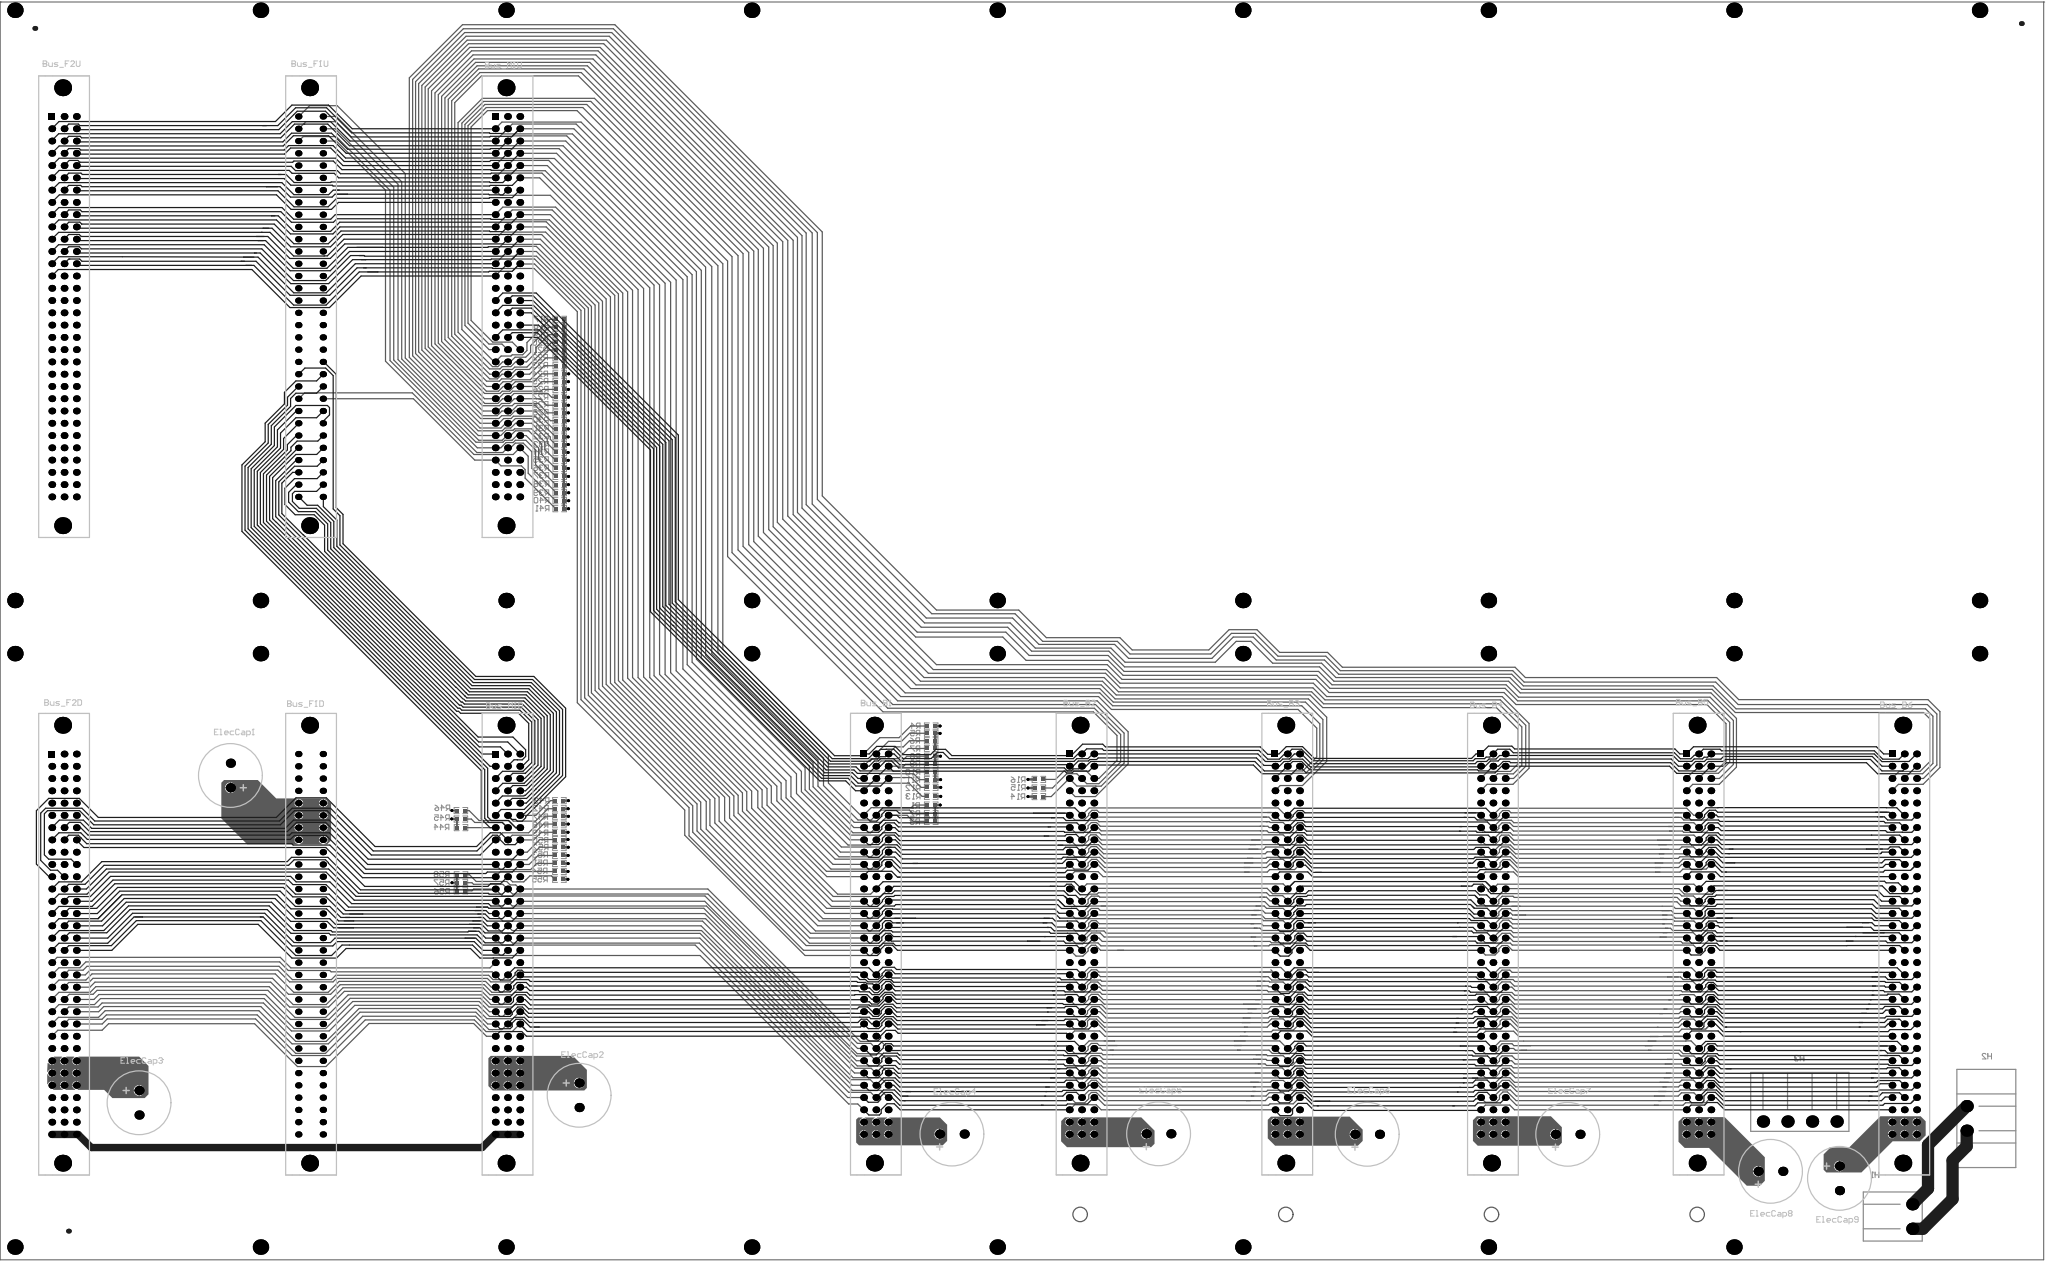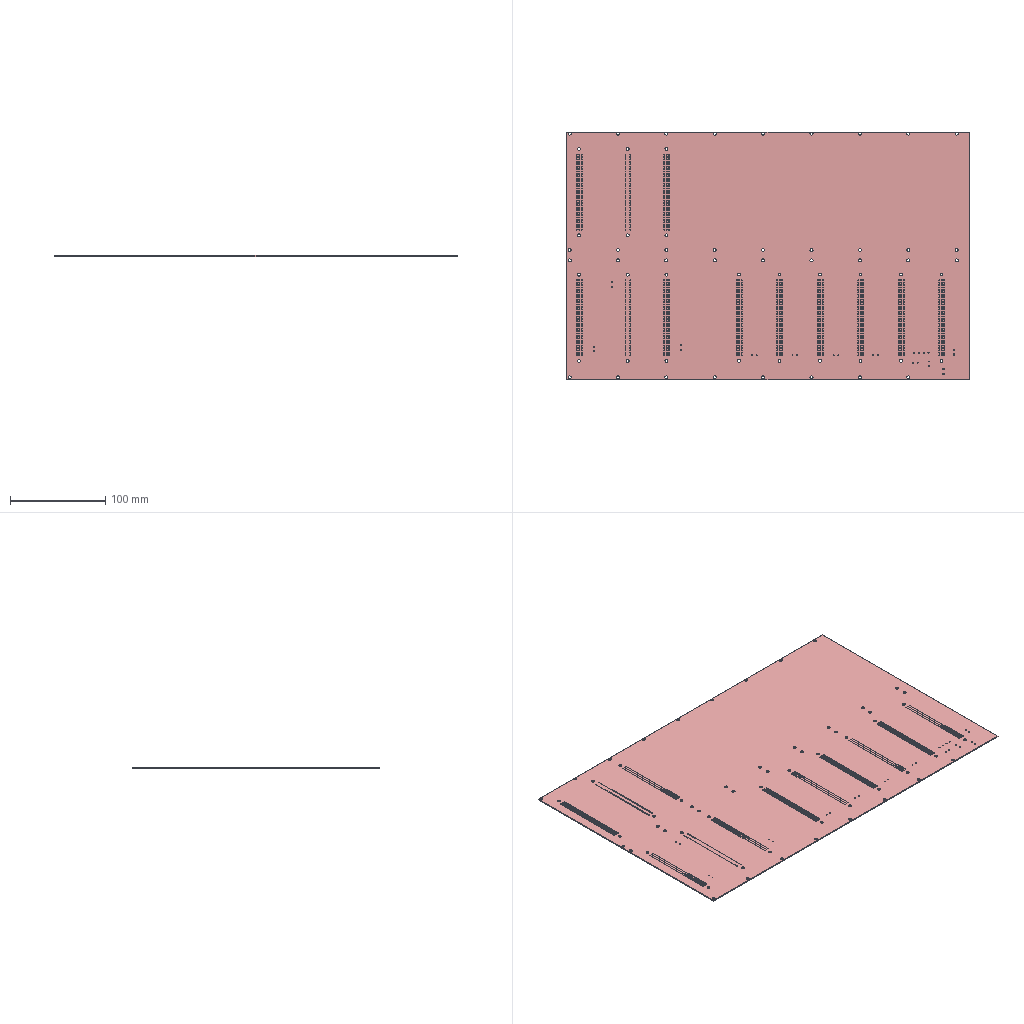Circuit board layout | Altium Designer | box 422.7 x 260.4 x 1.1 mm
Layer stack:
# Altium Designer layer stack of  (unit mm; dielectric type: 0 none, 1 core, 2 prepreg, 3 surface material)
index,name,kind,layer,copper_thickness_mm,dielectric_type,dielectric_thickness_mm,dielectric_material,dielectric_constant
0,TopPaste,other,,,,,,
1,TopOverlay,other,,,,,,
2,TopSolder,dielectric,,,3,0.0102,Solder Resist,3.5
3,TopLayer,copper,TopLayer,0.0356,,,,
4,Dielectric1,dielectric,,,1,0.32,FR-4,4.8
5,InternalPlane1,copper,InternalPlane1,0.0356,,,,
6,Dielectric2,dielectric,,,2,0.32,FR-4,4.8
7,InternalPlane2,copper,InternalPlane2,0.0356,,,,
8,Dielectric3,dielectric,,,1,0.32,FR-4,4.8
9,BottomLayer,copper,BottomLayer,0.0356,,,,
10,BottomSolder,dielectric,,,3,0.0102,Solder Resist,3.5
11,BottomOverlay,other,,,,,,
12,BottomPaste,other,,,,,,
# drill layer pairs: low layer,high layer
drill_pair,TopLayer,BottomLayer
Part placement:
Designator,Comment,Layer,Footprint,Center-X(mm),Center-Y(mm),Rotation
ElecCap9,1000uF/35V,TopLayer,1000UF/35V,275.819,16.866,90
ElecCap8,1000uF/35V,TopLayer,1000UF/35V,261.552,18.321,180
ElecCap7,1000uF/35V,TopLayer,1000UF/35V,219.608,25.984,180
ElecCap6,1000uF/35V,TopLayer,1000UF/35V,178.13,25.984,180
ElecCap5,1000uF/35V,TopLayer,1000UF/35V,134.976,26.086,180
ElecCap4,1000uF/35V,TopLayer,1000UF/35V,92.227,26.035,180
ElecCap3,1000uF/35V,TopLayer,1000UF/35V,-75.921,32.512,90
ElecCap2,1000uF/35V,TopLayer,1000UF/35V,15.113,34.061,90
ElecCap1,1000uF/35V,TopLayer,1000UF/35V,-57.023,100.254,270
Bus_F2U,OUPIIN Header32*3,TopLayer,OUPIINBUS32*3_ZHILI,-91.43,197.283,0
Bus_F2D,OUPIIN Header32*3,TopLayer,OUPIINBUS32*3_ZHILI,-91.43,65.324,0
Bus_M1D,OUPIIN Header32*3,TopLayer,OUPIINBUS32*3_ZHILI,0.3,65.324,360
Bus_M1U,OUPIIN Header32*3,TopLayer,OUPIINBUS32*3_ZHILI,0.3,197.283,360
Bus_B1,OUPIIN Header32*3,TopLayer,OUPIINBUS32*3_ZHILI,76.495,65.343,360
Bus_B2,OUPIIN Header32*3,TopLayer,OUPIINBUS32*3_ZHILI,119.045,65.343,360
Bus_B3,OUPIIN Header32*3,TopLayer,OUPIINBUS32*3_ZHILI,161.59,65.343,360
Bus_B4,OUPIIN Header32*3,TopLayer,OUPIINBUS32*3_ZHILI,204.135,65.343,360
Bus_B5,OUPIIN Header32*3,TopLayer,OUPIINBUS32*3_ZHILI,246.68,65.343,360
Bus_B6,OUPIIN Header32*3,TopLayer,OUPIINBUS32*3_ZHILI,289.225,65.343,360
Bus_F1U,CON64,TopLayer,OUPIINBUS32*2_ZHILI,-40.34,197.283,360
Bus_F1D,CON64,TopLayer,OUPIINBUS32*2_ZHILI,-40.34,65.324,360
R1,10k,BottomLayer,0603,87.935,94.132,180
R2,10k,BottomLayer,0603,87.935,92.38,360
R3,10k,BottomLayer,0603,87.935,90.754,180
R4,10k,BottomLayer,0603,87.935,110.49,180
R5,10k,BottomLayer,0603,87.935,108.991,360
R6,10k,BottomLayer,0603,87.935,107.442,180
R7,10k,BottomLayer,0603,87.935,105.842,180
R8,10k,BottomLayer,0603,87.935,104.242,0
R9,10k,BottomLayer,0603,87.935,102.565,180
R10,10k,BottomLayer,0603,87.935,100.965,180
R11,10k,BottomLayer,0603,87.935,99.39,180
R12,10k,BottomLayer,0603,87.935,97.79,0
R13,10k,BottomLayer,0603,87.935,95.936,180
R14,10k,BottomLayer,0603,110.211,95.885,360
R15,10k,BottomLayer,0603,110.211,97.663,180
R16,10k,BottomLayer,0603,110.211,99.441,360
R17,10k,BottomLayer,0603,11.1,194.666,180
R18,10k,BottomLayer,0603,11.1,193.065,0
R19,10k,BottomLayer,0603,11.1,191.491,180
R20,10k,BottomLayer,0603,11.1,189.916,180
R21,10k,BottomLayer,0603,11.1,188.316,360
R22,10k,BottomLayer,0603,11.1,186.69,180
R23,10k,BottomLayer,0603,11.1,185.064,180
R24,10k,BottomLayer,0603,11.1,183.388,360
R25,10k,BottomLayer,0603,11.1,181.762,180
R26,10k,BottomLayer,0603,11.1,180.162,180
R27,10k,BottomLayer,0603,11.1,178.537,0
R28,10k,BottomLayer,0603,11.1,176.886,180
R29,10k,BottomLayer,0603,11.1,175.311,180
R30,10k,BottomLayer,0603,11.1,173.685,0
R31,10k,BottomLayer,0603,11.1,171.983,180
R32,10k,BottomLayer,0603,11.1,170.332,180
R33,10k,BottomLayer,0603,11.1,168.732,0
R34,10k,BottomLayer,0603,11.1,167.107,180
R35,10k,BottomLayer,0603,11.1,165.481,180
R36,10k,BottomLayer,0603,11.1,163.805,360
R37,10k,BottomLayer,0603,11.1,162.154,180
R38,10k,BottomLayer,0603,11.1,160.452,180
R39,10k,BottomLayer,0603,11.1,158.775,360
R40,10k,BottomLayer,0603,11.1,157.124,180
R41,10k,BottomLayer,0603,11.1,155.473,180
R42,10k,BottomLayer,0603,11.024,93.37,360
R43,10k,BottomLayer,0603,11.024,95.047,180
R44,10k,BottomLayer,0603,-9.322,89.459,360
R45,10k,BottomLayer,0603,-9.347,91.237,180
R46,10k,BottomLayer,0603,-9.347,92.989,360
R47,10k,BottomLayer,0603,11.024,91.821,180
R48,10k,BottomLayer,0603,11.024,90.195,360
R49,10k,BottomLayer,0603,11.024,88.494,180
R50,10k,BottomLayer,0603,11.024,86.995,180
R51,10k,BottomLayer,0603,11.024,82.042,180
R52,10k,BottomLayer,0603,11.024,85.395,360
R53,10k,BottomLayer,0603,11.024,83.693,180
R54,10k,BottomLayer,0603,11.024,80.391,180
R55,10k,BottomLayer,0603,11.024,78.765,360
R56,10k,BottomLayer,0603,-9.347,76.378,360
R57,10k,BottomLayer,0603,-9.347,78.054,180
R58,10k,BottomLayer,0603,-9.322,79.705,360
H3,Header4,BottomLayer,EDGCON_4p_5.08mm,267.614,28.626,360
H2,Header2,BottomLayer,EDGCON_2p_5.08mm_ear,302.133,29.261,270
H1,Header2,BottomLayer,EDGCon_2p_5.08mm,290.906,8.966,90
Pad and via stacks:
# Altium Designer via and pad stacks of  (unit mm). Each distinct definition once, with the count of objects using it.
# via: kind,start_layer,end_layer,hole_mm,diameter_mm,mode(0 simple;1 top-mid-bottom;2 full stack),diameter_per_layer,count,example_net
# pad: kind,layer,hole_mm,hole_type(0 round;1 square;2 slot),plating,top_size,top_shape(1 round;2 rect;3 octagon;9 rounded rect),mid_size,bottom_size,mode,footprint,size_per_layer,count,example
pad,MultiLayer,1.016,0,plated,1.9x1.9,1,1.9x1.9,1.9x1.9,0,1000UF/35V,,18,ElecCap1.1
pad,MultiLayer,0.9652,0,plated,1.397x1.397,1,1.397x1.397,1.397x1.397,0,OUPIINBUS32*3_ZHILI,,950,Bus_B6.A4
pad,MultiLayer,3,0,plated,3.5x3.5,1,3.5x3.5,3.5x3.5,0,OUPIINBUS32*3_ZHILI,,20,Bus_B6.0
pad,MultiLayer,0.9652,0,plated,1.397x1.397,2,1.397x1.397,1.397x1.397,0,OUPIINBUS32*3_ZHILI,,10,Bus_B6.A1
pad,MultiLayer,0.9652,0,plated,1.524x1.27,1,1.524x1.27,1.524x1.27,0,OUPIINBUS32*2_ZHILI,,128,Bus_F1D.A9
pad,MultiLayer,3,0,plated,3.5x3.5,1,3.5x3.5,3.5x3.5,0,OUPIINBUS32*2_ZHILI,,4,Bus_F1D.0
pad,MultiLayer,3.2,0,plated,3.2x3.2,1,3.2x3.2,3.2x3.2,0,,,35,1
pad,MultiLayer,1.295,0,plated,2.54x2.54,1,2.54x2.54,2.54x2.54,0,EDGCON_4p_5.08mm,,4,H3.3
pad,MultiLayer,1.295,0,plated,2.54x2.54,1,2.54x2.54,2.54x2.54,0,EDGCON_2p_5.08mm_ear,,2,H2.2
pad,MultiLayer,1.295,0,plated,2.54x2.54,1,2.54x2.54,2.54x2.54,0,EDGCon_2p_5.08mm,,2,H1.2
pad,BottomLayer,0,0,plated,0.635x0.8128,2,0.635x0.8128,0.635x0.8128,0,0603,,116,R1.1
pad,BottomLayer,0,0,plated,1x1,1,1x1,1x1,0,,,3,0
pad,TopLayer,0,0,plated,1x1,1,1x1,1x1,0,,,3,0
via,TopLayer,BottomLayer,0.3048,0.6096,0,,42,GND
Copper pours:
name,layer,net,type(0 solid;1 hatched;2 none)
TopLayer-No Net,BottomLayer,+5V,0
TopLayer-No Net,BottomLayer,+5V,0
TopLayer-No Net,BottomLayer,+5V,0
TopLayer-No Net,BottomLayer,+5V,0
TopLayer-No Net,BottomLayer,+5V,0
TopLayer-No Net,BottomLayer,+5V,0
TopLayer-No Net,BottomLayer,+5V,0
TopLayer-No Net,BottomLayer,+5V,0
TopLayer-No Net,BottomLayer,+5V,0
Design rules, without the lines most boards share:
# Altium Designer design rules of  (exported by Altium Designer, unit mm)
# columns: name | kind | enabled | priority | scope1 | scope2 | descriptor | typed fields (field=value)
DiffPairsRouting | 51 | enabled | 1 | All | All | Differential Pairs Uncoupled Length using the Gap Constraints (Min=0.254mm) (Max=0.254mm) (Prefered=0.254mm)  and Width Constraints (Min=0.381mm) (Max=0.381mm) (Prefered=0.381mm) (All) |
Height | 50 | enabled | 1 | All | All | Height Constraint (Min=0mm) (Max=25.4mm) (Prefered=12.7mm) (All) | min_height=0 max_height=25.4
Clearance | 0 | enabled | 1 | All | All | Clearance Constraint (Gap=0.152mm) (All),(All) | gap=0.1524
PlaneConnect | 6 | enabled | 1 | All | All | Power Plane Connect Rule(Direct Connect )(Expansion=0.508mm) (Conductor Width=0.254mm) (Air Gap=0.254mm) (Entries=4) (All) | relief_conductor_width=0.254 relief_entries=4 relief_expansion=0.508
PlaneClearance | 12 | enabled | 1 | All | All | Power Plane Clearance (Clearance =0.508mm) (All) | clearance=0.508
PolygonConnect | 20 | enabled | 1 | All | All | Polygon Connect Rule(Relief Connect )(Conductor Width=0.254mm) (Relief Angle=90 Angle) (Entries=4) (Air Gap Width=0.254mm) (All),(All) | connect_style(0=relief,1=direct,2=none)=0 relief_conductor_width=0.254 relief_entries=4
Width | 2 | enabled | 1 | All | All | Width Constraint (Min=0.254mm) (Max=25.4mm) (Preferred=0.254mm) (All) |
RoutingCorners | 10 | enabled | 1 | All | All | Routing Corners (Style=45-Degree) (Min Setback=2.54mm) (Max Setback=2.54mm) (All) |
RoutingVias | 11 | enabled | 1 | All | All | Routing Via (MinHoleWidth=0.305mm) (MaxHoleWidth=0.711mm) (PreferredHoleWidth=0.508mm) (MinWidth=0.61mm) (MaxWidth=1.27mm) (PreferedWidth=1.016mm) (All) | via_min_hole=0.3048 via_max_hole=0.7112 via_preferred_diameter=1.016 via_preferred_hole=0.508
PasteMaskExpansion | 14 | enabled | 1 | All | All | Paste Mask Expansion (Expansion =0mm) (All) | expansion=0
SolderMaskExpansion | 13 | enabled | 1 | All | All | Solder Mask Expansion (Expansion =0.102mm) (All) | expansion=0.1016
TestPointUsage | 44 | enabled | 1 | All | All | Fabrication Testpoint Usage (Valid =One Required, Allow multiple per net=No) (All) |
Testpoint | 43 | enabled | 1 | All | All | Fabrication Testpoint Style (Under Component=Yes) (All) |
HoleSize | 42 | enabled | 1 | All | All | Hole Size Constraint (Min=0.025mm) (Max=2.54mm) (All) |
ComponentClearance | 24 | disabled | 1 | All | All | Component Clearance Constraint ( Horizontal Gap = 0.254mm, Vertical Gap = 0.254mm ) (Disabled)(All),(All)  | gap=0.254
HoleToHoleClearance | 52 | enabled | 1 | All | All | Hole To Hole Clearance (Gap=0.254mm) (All),(All) | gap=0.254
MinimumSolderMaskSliver | 53 | enabled | 1 | All | All | Minimum Solder Mask Sliver (Gap=0.254mm) (All),(All) |
SilkscreenOverComponentPads | 54 | enabled | 1 | IsPad | All | Silk To Solder Mask (Clearance=0.254mm) (IsPad),(All) |
SilkToSilkClearance | 55 | enabled | 1 | All | All | Silk to Silk (Clearance=0.254mm) (All),(All) |
NetAntennae | 56 | enabled | 1 | All | All | Net Antennae (Tolerance=0mm) (All) |
Classes set for this board:
# Altium Designer classes of  (member kind: 0 net, 1 component, 2 from-to, 3 pad, 4 layer, 5 differential pair, 6 design channel, 7 polygon, 8 structure, 9 xSignal)
# columns: class name | member kind | superclass | members
All From-Tos | 0 | yes |